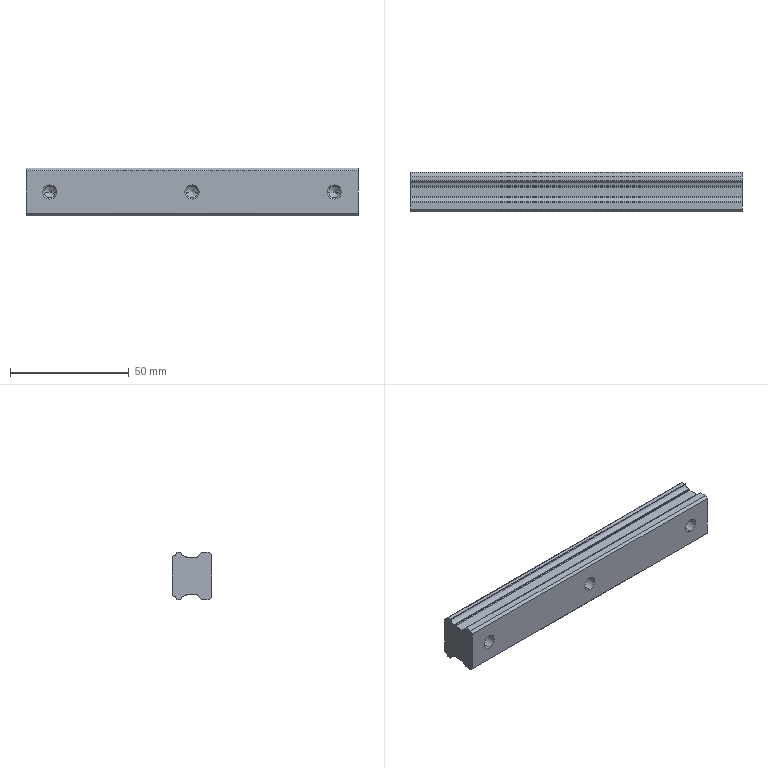Part | STEP file | J454-EBZ05-99-04-Part-1-4 | 1 solid | 60 faces | box 140 x 16.5 x 20 mm | volume 40392 mm3 | cylinder 32 | plane 16 | cone 12 | commonest cylinder face diameters 0.4 x9 4.917 x6 6 x6 3.604 x5 1 x4 0.5 x2